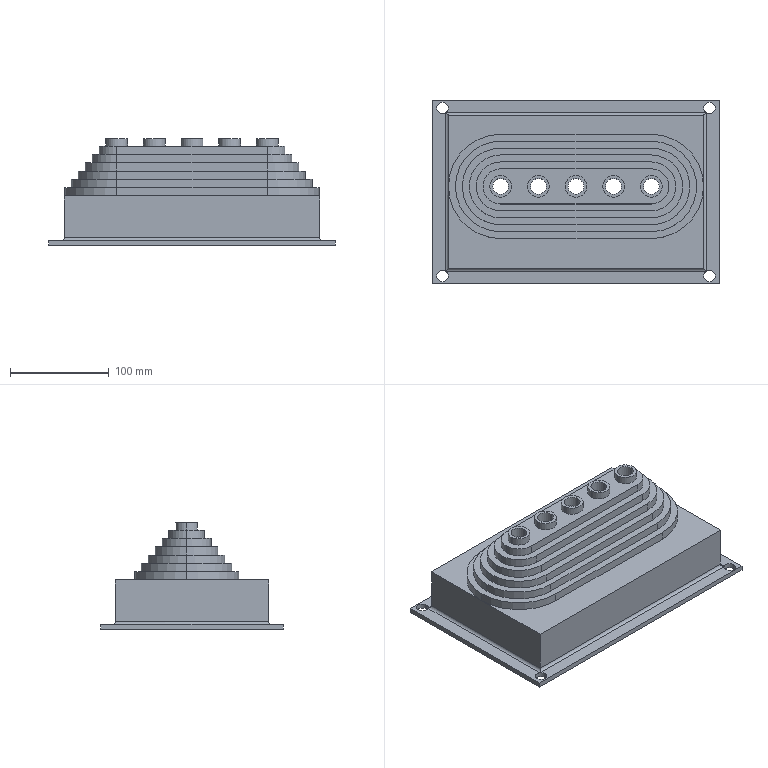Part | SolidWorks | features ICE 18, BossThin 5, LPattern 3, RefAxis 2, Extrusion 1, Fillet 1 | 1 solid | 127 faces | box 290 x 185 x 108 mm | volume 384373 mm3 | cylinder 68 | plane 59 | commonest cylinder face diameters 16 x10 22 x10 12 x8 6 x4 29.6 x3 35.6 x3